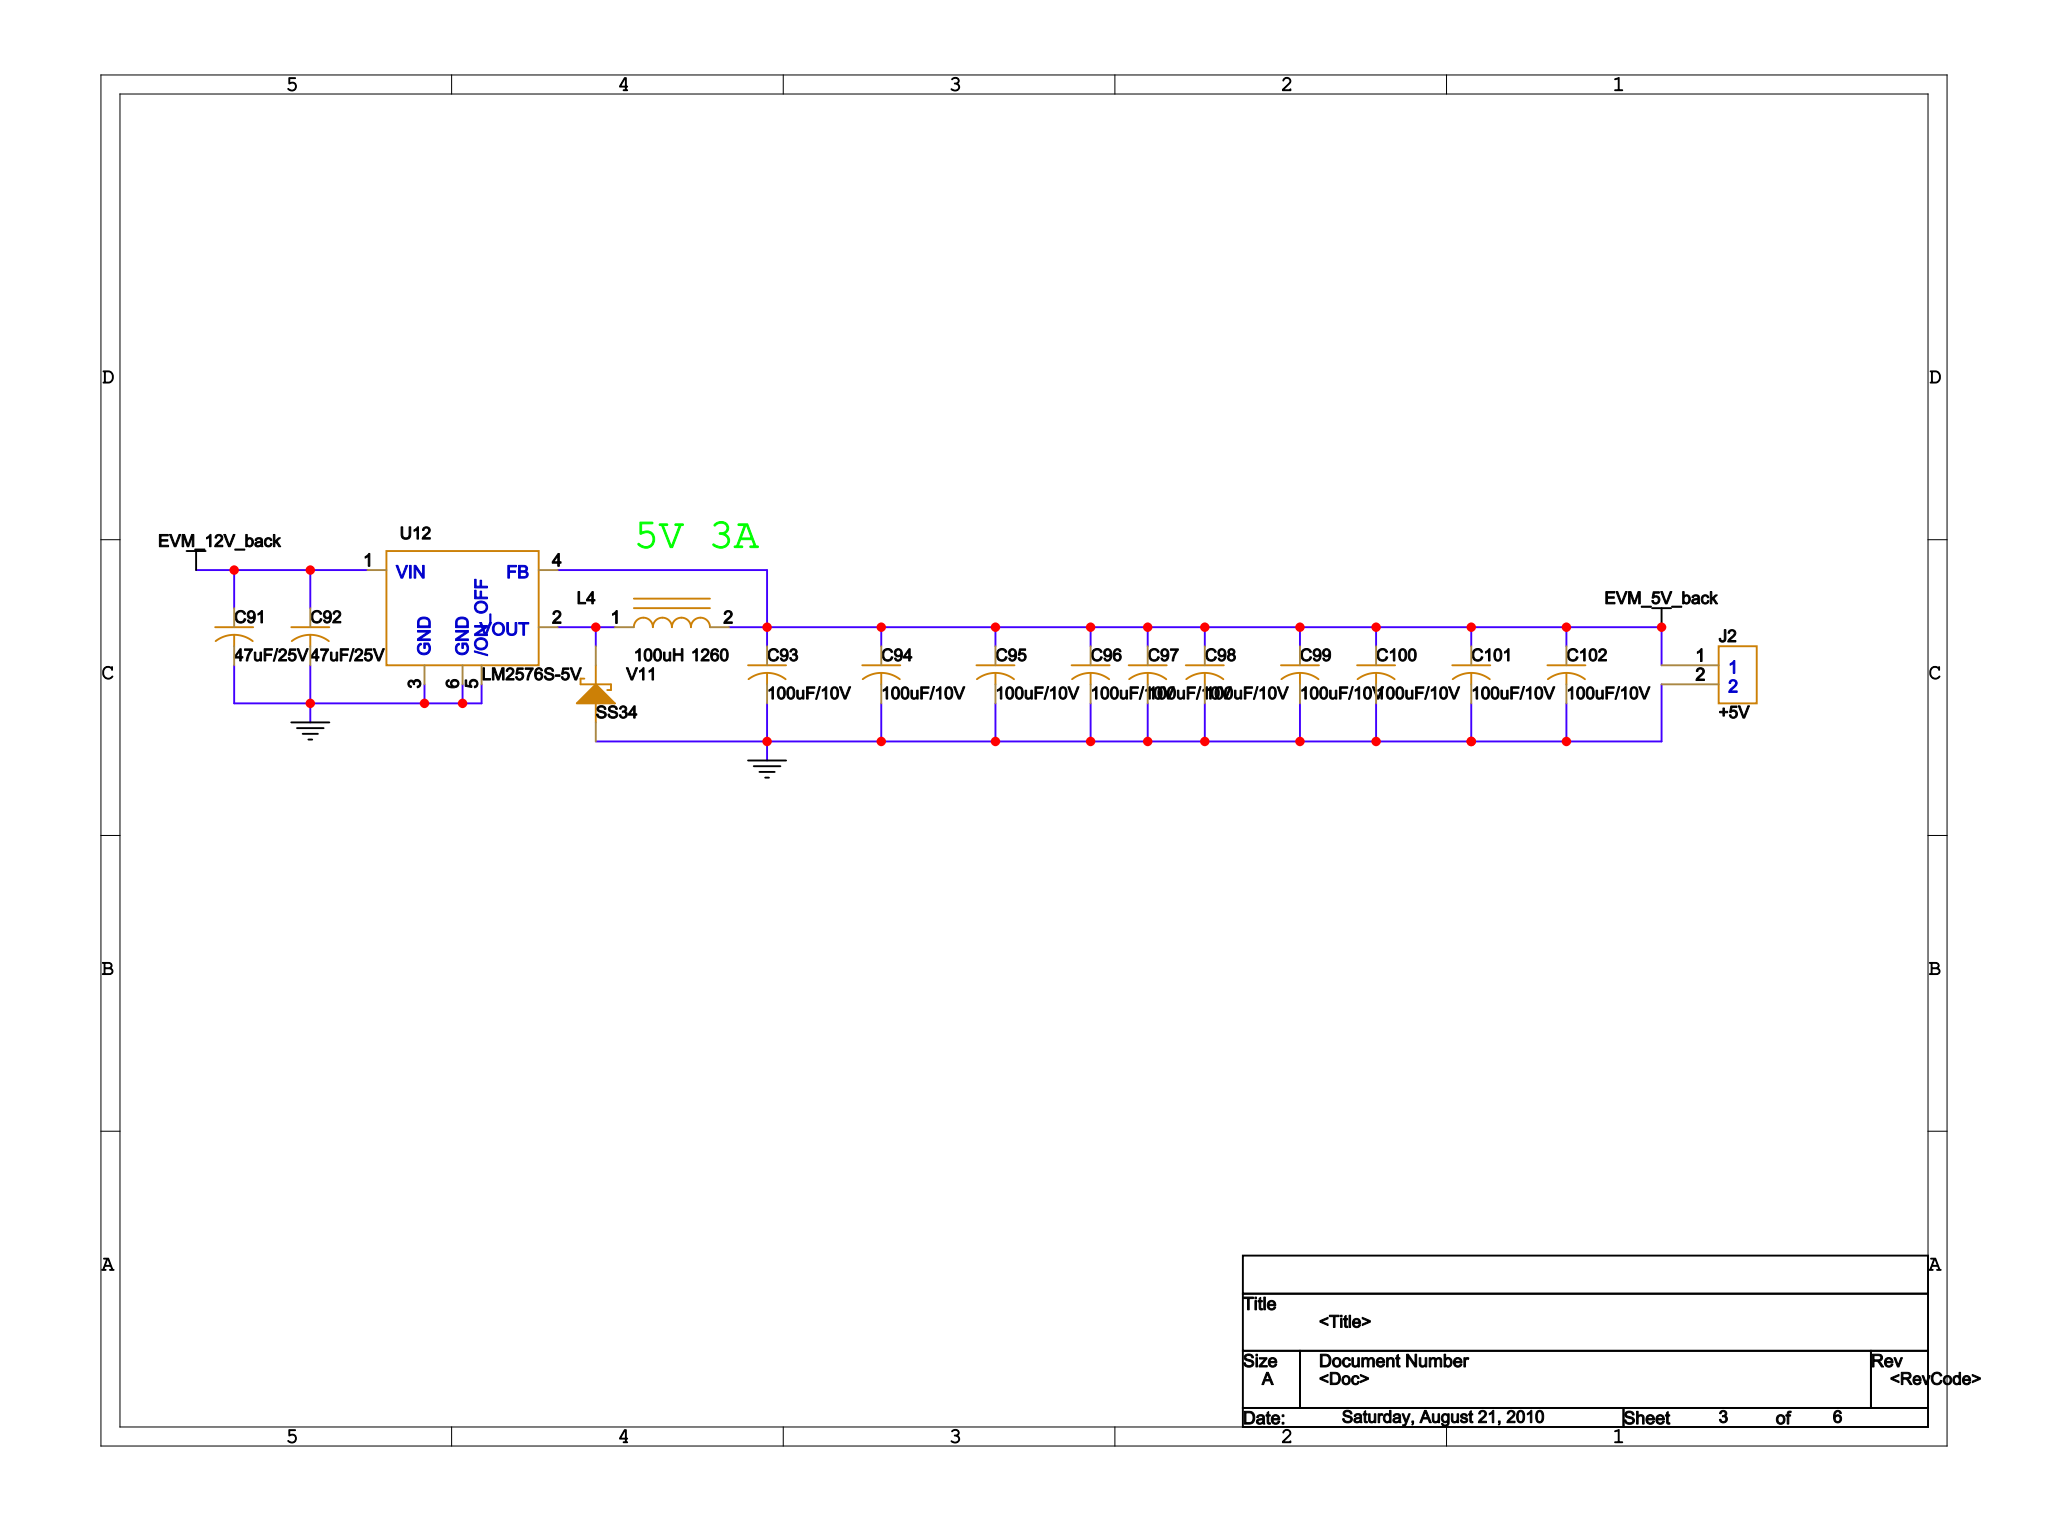Circuit board | Cadence Allegro | 241 parts | 116 nets | one sheet of the schematic
Parts on this sheet (reference | value | footprint):
C91 | 47uF/25V | C1210
C92 | 47uF/25V | C1210
C93 | 100uF/10V | C1210
C94 | 100uF/10V | C1210
C95 | 100uF/10V | C1210
C96 | 100uF/10V | C1210
C97 | 100uF/10V | C1210
C98 | 100uF/10V | C1210
C99 | 100uF/10V | C1210
C100 | 100uF/10V | C1210
C101 | 100uF/10V | C1210
C102 | 100uF/10V | C1210
J2 | +5V | HDR2MM54_1X2
L4 | 100uH | L-12X14X8
U12 | LM2576S-5V | TO-263
V11 | SS34 | DO214AB
Nets of these parts (net: part-pin ...):
GND: C91-2 C92-2 C93-2 C94-2 C95-2 C96-2 C97-2 C98-2 C99-2 C100-2 C101-2 C102-2 J2-2 U12-3 U12-5 U12-6 V11-2
EVM_5V_BACK: C93-1 C94-1 C95-1 C96-1 C97-1 C98-1 C99-1 C100-1 C101-1 C102-1 J2-1 L4-2 U12-4
EVM_12V_BACK: C91-1 C92-1 U12-1
N19149447: L4-1 U12-2 V11-1